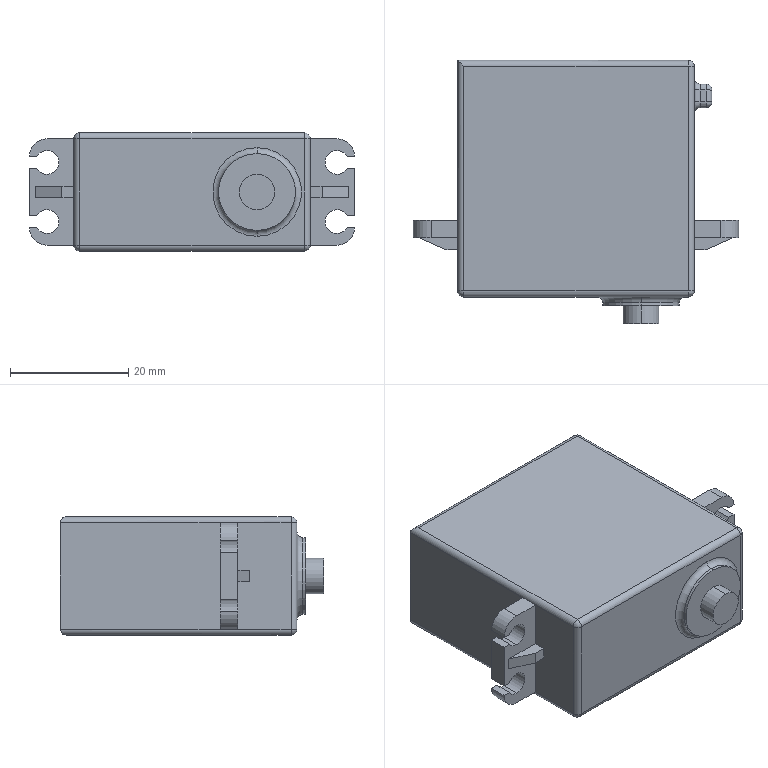Part | STEP file | Servo single shaft | 1 solid | 100 faces | box 55 x 44.5 x 20 mm | volume 32938 mm3 | cylinder 43 | plane 41 | sphere 10 | torus 6 | commonest cylinder face diameters 2 x23 4 x12 6 x6 13 x2